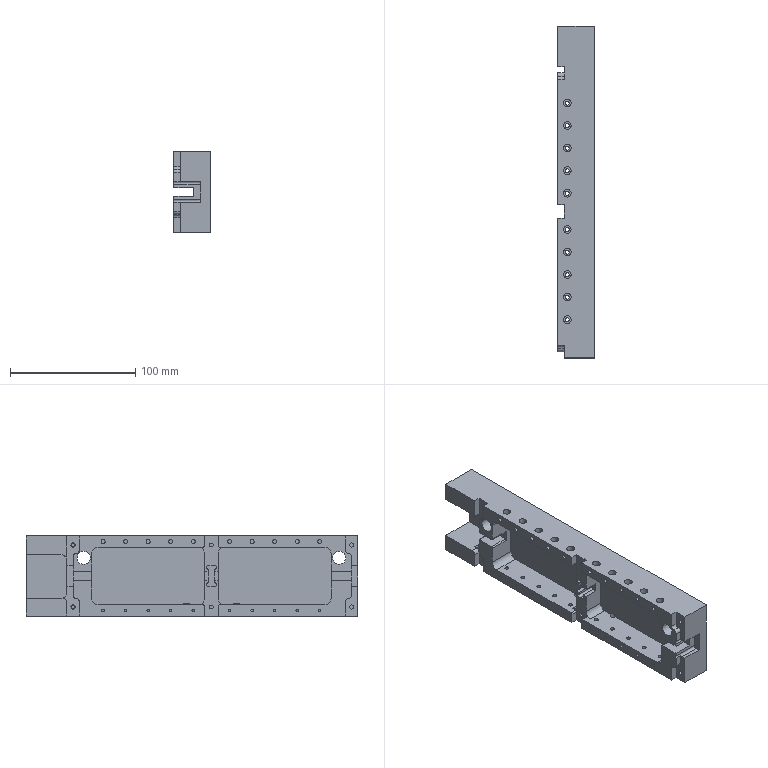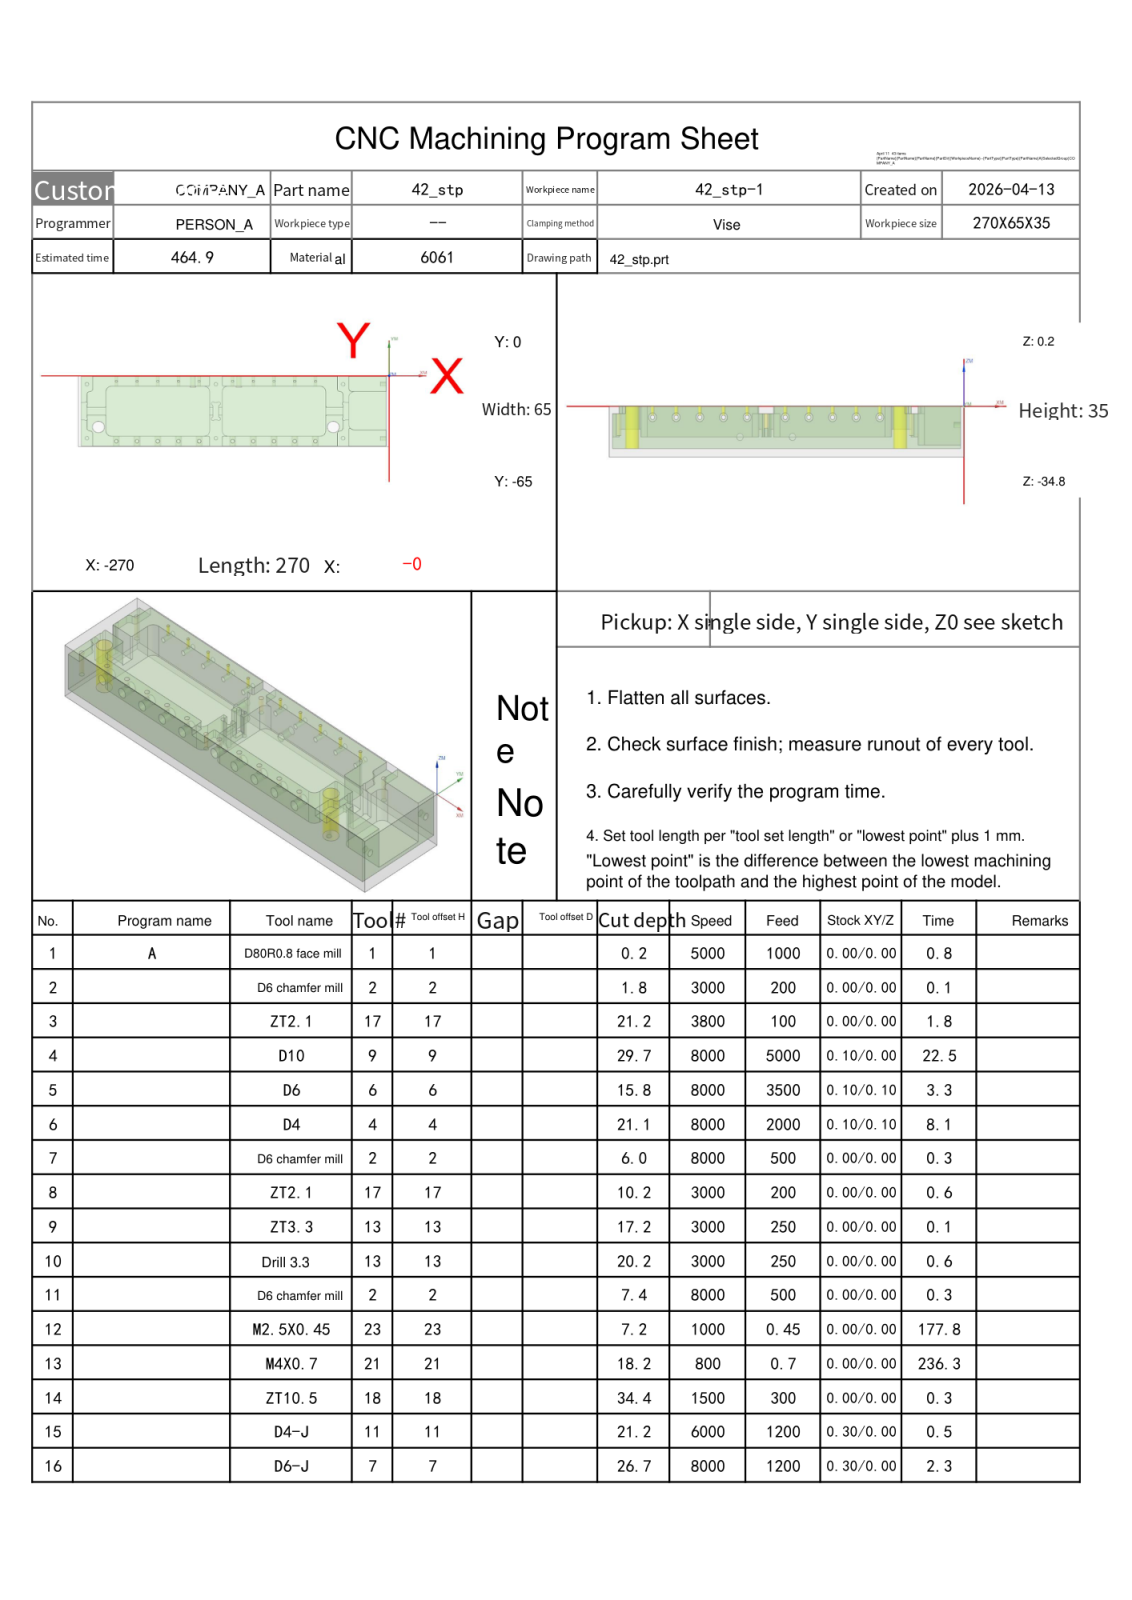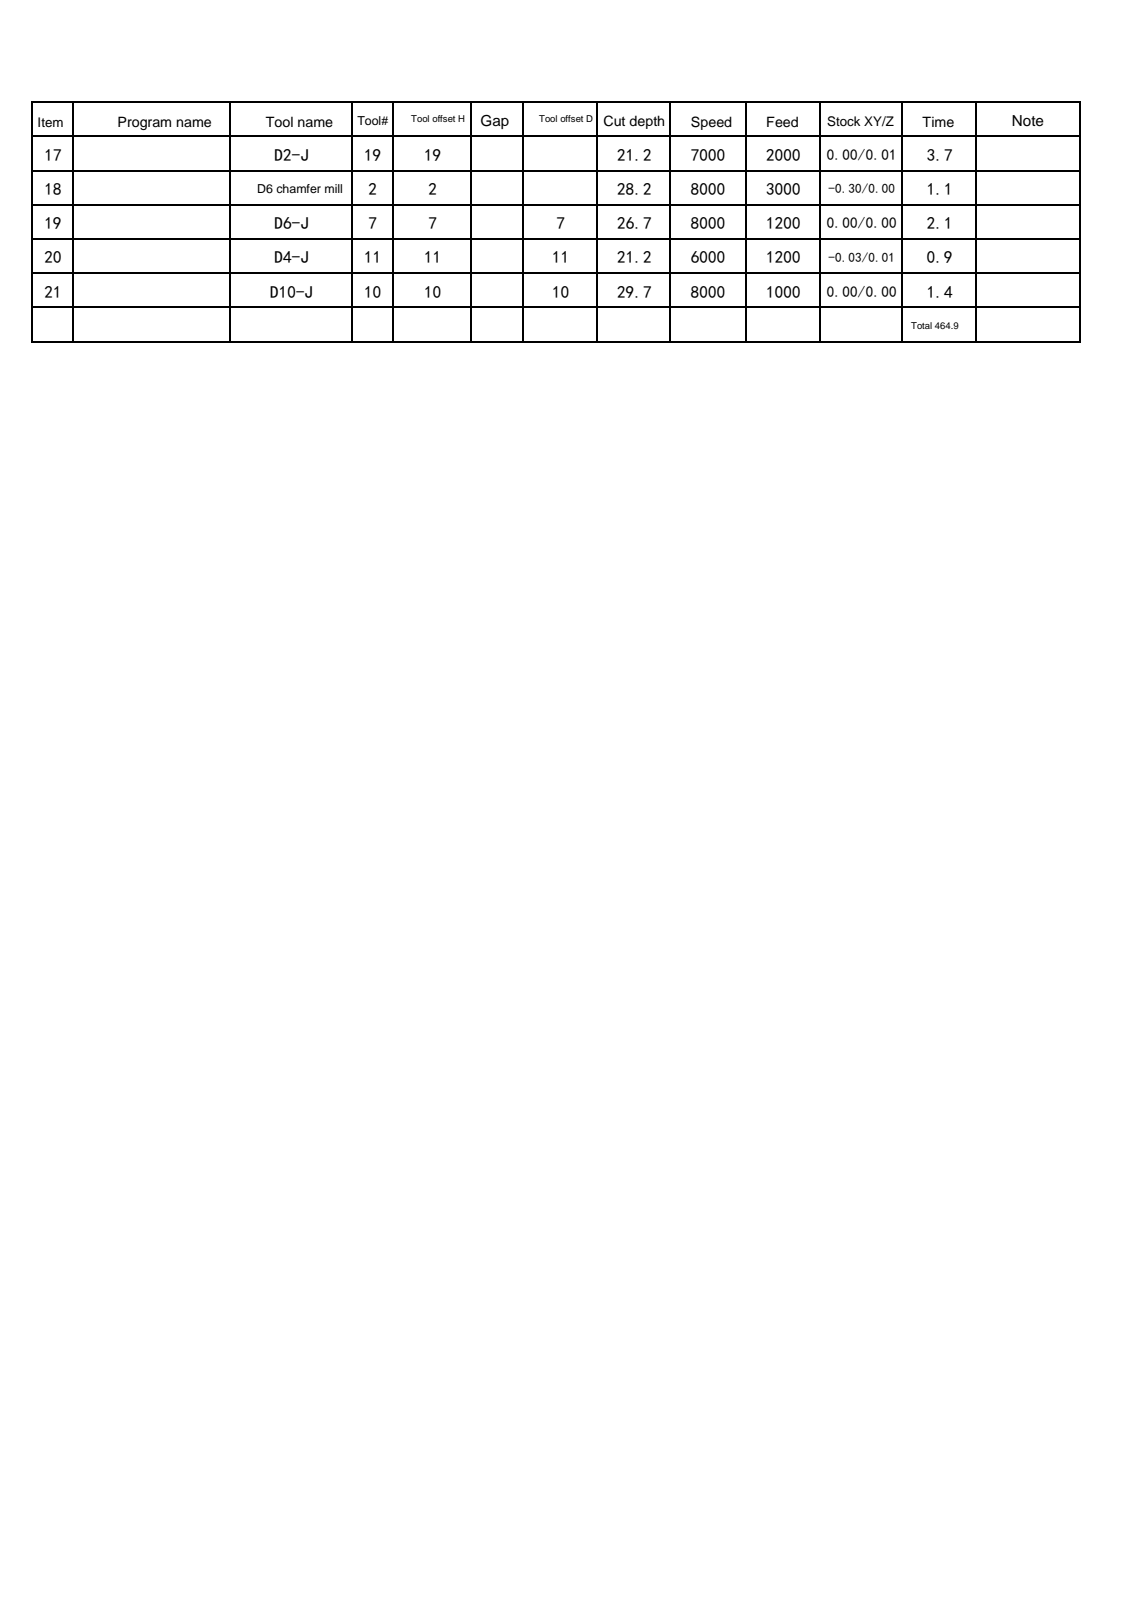NC program | NX | posted by the shop | part box 29 x 265 x 64 mm
Lines 6965 to 7681 of 41846:
N6 T04 M06
(D4  D=4. R=0. H=04 ce=0.10 di=0.10)
G00 G90 G54 X-150.05 Y-30.444 M03 S8000
G43 H04 Z20.
M08
Z-4.
G01 X-150.033 Y-26.941 Z-4.184 F2000.
X-149.901 Y-26.57 Z-4.204
X-151.099 Z-4.267
X-150.95 Y-27.178 Z-4.3
X-150.967 Y-38.059 Z-4.87
X-151.099 Y-38.43 Z-4.891
X-149.901 Z-4.954
X-150.033 Y-38.059 Z-4.974
X-150.05 Y-37.963 Z-4.979
Y-37.569 Z-5.
Y-27.431 Z-5.077
G02 X-149.901 Y-26.57 Z-5.084 I2.57 J0.0
G01 X-151.099 Z-5.093
G02 X-150.999 Y-26.93 Z-5.096 I-2.421 J-.861
X-150.95 Y-27.431 Z-5.099 I-2.521 J-.501
G01 Y-37.569 Z-5.176
G02 X-151.099 Y-38.43 Z-5.183 I-2.57 J0.0
G01 X-149.901 Z-5.192
G02 X-150.05 Y-37.569 Z-5.199 I2.421 J.861
G01 Y-27.431 Z-5.276
G02 X-149.901 Y-26.57 Z-5.282 I2.57 J0.0
G01 X-151.099 Z-5.291
G02 X-150.999 Y-26.93 Z-5.294 I-2.421 J-.861
X-150.95 Y-27.431 Z-5.298 I-2.521 J-.501
G01 Y-37.569 Z-5.375
G02 X-151.099 Y-38.43 Z-5.382 I-2.57 J0.0
G01 X-149.901 Z-5.391
G02 X-150.05 Y-37.569 Z-5.398 I2.421 J.861
G01 Y-27.431 Z-5.474
G02 X-149.901 Y-26.57 Z-5.481 I2.57 J0.0
G01 X-151.099 Z-5.49
G02 X-150.999 Y-26.93 Z-5.493 I-2.421 J-.861
X-150.95 Y-27.431 Z-5.497 I-2.521 J-.501
G01 Y-37.569 Z-5.574
G02 X-151.099 Y-38.43 Z-5.58 I-2.57 J0.0
G01 X-149.901 Z-5.59
G02 X-150.05 Y-37.569 Z-5.596 I2.421 J.861
G01 Y-27.431 Z-5.673
G02 X-149.901 Y-26.57 Z-5.68 I2.57 J0.0
G01 X-151.099 Z-5.689
G02 X-150.999 Y-26.93 Z-5.692 I-2.421 J-.861
X-150.95 Y-27.431 Z-5.696 I-2.521 J-.501
G01 Y-37.569 Z-5.773
G02 X-151.099 Y-38.43 Z-5.779 I-2.57 J0.0
G01 X-149.901 Z-5.788
G02 X-150.05 Y-37.569 Z-5.795 I2.421 J.861
G01 Y-27.431 Z-5.872
G02 X-149.901 Y-26.57 Z-5.879 I2.57 J0.0
G01 X-151.099 Z-5.888
G02 X-150.999 Y-26.93 Z-5.891 I-2.421 J-.861
X-150.95 Y-27.431 Z-5.894 I-2.521 J-.501
G01 Y-37.569 Z-5.971
G02 X-151.099 Y-38.43 Z-5.978 I-2.57 J0.0
G01 X-149.901 Z-5.987
G02 X-150.05 Y-37.569 Z-5.994 I2.421 J.861
G01 Y-27.431 Z-6.071
G02 X-149.901 Y-26.57 Z-6.077 I2.57 J0.0
G01 X-151.099 Z-6.086
G02 X-150.999 Y-26.93 Z-6.089 I-2.421 J-.861
X-150.95 Y-27.431 Z-6.093 I-2.521 J-.501
G01 Y-37.569 Z-6.17
G02 X-151.099 Y-38.43 Z-6.177 I-2.57 J0.0
G01 X-149.901 Z-6.186
G02 X-150.05 Y-37.569 Z-6.193 I2.421 J.861
G01 Y-27.431 Z-6.269
G02 X-149.901 Y-26.57 Z-6.276 I2.57 J0.0
G01 X-151.099 Z-6.285
G02 X-150.999 Y-26.93 Z-6.288 I-2.421 J-.861
X-150.95 Y-27.431 Z-6.292 I-2.521 J-.501
G01 Y-37.569 Z-6.369
G02 X-151.099 Y-38.43 Z-6.375 I-2.57 J0.0
G01 X-149.901 Z-6.385
G02 X-150.05 Y-37.569 Z-6.391 I2.421 J.861
G01 Y-27.431 Z-6.468
G02 X-149.901 Y-26.57 Z-6.475 I2.57 J0.0
G01 X-151.099 Z-6.484
G02 X-150.999 Y-26.93 Z-6.487 I-2.421 J-.861
X-150.95 Y-27.431 Z-6.491 I-2.521 J-.501
G01 Y-37.569 Z-6.568
G02 X-151.099 Y-38.43 Z-6.574 I-2.57 J0.0
G01 X-149.901 Z-6.583
G02 X-150.05 Y-37.569 Z-6.59 I2.421 J.861
G01 Y-27.431 Z-6.667
G02 X-149.901 Y-26.57 Z-6.674 I2.57 J0.0
G01 X-151.099 Z-6.683
G02 X-150.999 Y-26.93 Z-6.686 I-2.421 J-.861
X-150.95 Y-27.431 Z-6.689 I-2.521 J-.501
G01 Y-37.569 Z-6.766
G02 X-151.099 Y-38.43 Z-6.773 I-2.57 J0.0
G01 X-149.901 Z-6.782
G02 X-150.05 Y-37.569 Z-6.789 I2.421 J.861
G01 Y-27.431 Z-6.866
G02 X-149.901 Y-26.57 Z-6.872 I2.57 J0.0
G01 X-151.099 Z-6.881
G02 X-150.999 Y-26.93 Z-6.884 I-2.421 J-.861
X-150.95 Y-27.431 Z-6.888 I-2.521 J-.501
G01 Y-37.569 Z-6.965
G02 X-151.099 Y-38.43 Z-6.972 I-2.57 J0.0
G01 X-149.901 Z-6.981
G02 X-150.05 Y-37.569 Z-6.988 I2.421 J.861
G01 Y-27.431 Z-7.064
G02 X-149.901 Y-26.57 Z-7.071 I2.57 J0.0
G01 X-151.099 Z-7.08
G02 X-150.999 Y-26.93 Z-7.083 I-2.421 J-.861
X-150.95 Y-27.431 Z-7.087 I-2.521 J-.501
G01 Y-37.569 Z-7.164
G02 X-151.099 Y-38.43 Z-7.17 I-2.57 J0.0
G01 X-149.901 Z-7.18
G02 X-150.05 Y-37.569 Z-7.186 I2.421 J.861
G01 Y-27.431 Z-7.263
G02 X-149.901 Y-26.57 Z-7.27 I2.57 J0.0
G01 X-151.099 Z-7.279
G02 X-150.999 Y-26.93 Z-7.282 I-2.421 J-.861
X-150.95 Y-27.431 Z-7.286 I-2.521 J-.501
G01 Y-37.569 Z-7.363
G02 X-151.099 Y-38.43 Z-7.369 I-2.57 J0.0
G01 X-149.901 Z-7.378
G02 X-150.05 Y-37.569 Z-7.385 I2.421 J.861
G01 Y-27.431 Z-7.462
G02 X-149.901 Y-26.57 Z-7.469 I2.57 J0.0
G01 X-151.099 Z-7.478
G02 X-150.999 Y-26.93 Z-7.481 I-2.421 J-.861
X-150.95 Y-27.431 Z-7.484 I-2.521 J-.501
G01 Y-37.569 Z-7.561
G02 X-151.099 Y-38.43 Z-7.568 I-2.57 J0.0
G01 X-149.901 Z-7.577
G02 X-150.05 Y-37.569 Z-7.584 I2.421 J.861
G01 Y-27.431 Z-7.661
G02 X-149.901 Y-26.57 Z-7.667 I2.57 J0.0
G01 X-151.099 Z-7.676
G02 X-150.999 Y-26.93 Z-7.679 I-2.421 J-.861
X-150.95 Y-27.431 Z-7.683 I-2.521 J-.501
G01 Y-37.569 Z-7.76
G02 X-151.099 Y-38.43 Z-7.767 I-2.57 J0.0
G01 X-149.901 Z-7.776
G02 X-150.05 Y-37.569 Z-7.783 I2.421 J.861
G01 Y-27.431 Z-7.859
G02 X-149.901 Y-26.57 Z-7.866 I2.57 J0.0
G01 X-151.099 Z-7.875
G02 X-150.999 Y-26.93 Z-7.878 I-2.421 J-.861
X-150.95 Y-27.431 Z-7.882 I-2.521 J-.501
G01 Y-37.569 Z-7.959
G02 X-151.099 Y-38.43 Z-7.965 I-2.57 J0.0
G01 X-149.901 Z-7.975
G02 X-150.05 Y-37.569 Z-7.981 I2.421 J.861
G01 Y-27.431 Z-8.058
G02 X-149.901 Y-26.57 Z-8.065 I2.57 J0.0
G01 X-151.099 Z-8.074
G02 X-150.999 Y-26.93 Z-8.077 I-2.421 J-.861
X-150.95 Y-27.431 Z-8.081 I-2.521 J-.501
G01 Y-37.569 Z-8.158
G02 X-151.099 Y-38.43 Z-8.164 I-2.57 J0.0
G01 X-149.901 Z-8.173
G02 X-150.05 Y-37.569 Z-8.18 I2.421 J.861
G01 Y-27.431 Z-8.257
G02 X-149.901 Y-26.57 Z-8.264 I2.57 J0.0
G01 X-151.099 Z-8.273
G02 X-150.999 Y-26.93 Z-8.276 I-2.421 J-.861
X-150.95 Y-27.431 Z-8.279 I-2.521 J-.501
G01 Y-37.569 Z-8.356
G02 X-151.099 Y-38.43 Z-8.363 I-2.57 J0.0
G01 X-149.901 Z-8.372
G02 X-150.05 Y-37.569 Z-8.379 I2.421 J.861
G01 Y-27.431 Z-8.456
G02 X-149.901 Y-26.57 Z-8.462 I2.57 J0.0
G01 X-151.099 Z-8.471
G02 X-150.999 Y-26.93 Z-8.474 I-2.421 J-.861
X-150.95 Y-27.431 Z-8.478 I-2.521 J-.501
G01 Y-37.569 Z-8.555
G02 X-151.099 Y-38.43 Z-8.562 I-2.57 J0.0
G01 X-149.901 Z-8.571
G02 X-150.05 Y-37.569 Z-8.578 I2.421 J.861
G01 Y-27.431 Z-8.654
G02 X-149.901 Y-26.57 Z-8.661 I2.57 J0.0
G01 X-151.099 Z-8.67
G02 X-150.999 Y-26.93 Z-8.673 I-2.421 J-.861
X-150.95 Y-27.431 Z-8.677 I-2.521 J-.501
G01 Y-37.569 Z-8.754
G02 X-151.099 Y-38.43 Z-8.76 I-2.57 J0.0
G01 X-149.901 Z-8.77
G02 X-150.05 Y-37.569 Z-8.776 I2.421 J.861
G01 Y-27.431 Z-8.853
G02 X-149.901 Y-26.57 Z-8.86 I2.57 J0.0
G01 X-151.099 Z-8.869
G02 X-150.999 Y-26.93 Z-8.872 I-2.421 J-.861
X-150.95 Y-27.431 Z-8.876 I-2.521 J-.501
G01 Y-37.569 Z-8.953
G02 X-151.099 Y-38.43 Z-8.959 I-2.57 J0.0
G01 X-149.901 Z-8.968
G02 X-150.05 Y-37.569 Z-8.975 I2.421 J.861
G01 Y-27.431 Z-9.052
G02 X-149.901 Y-26.57 Z-9.059 I2.57 J0.0
G01 X-151.099 Z-9.068
G02 X-150.999 Y-26.93 Z-9.071 I-2.421 J-.861
X-150.95 Y-27.431 Z-9.074 I-2.521 J-.501
G01 Y-37.569 Z-9.151
G02 X-151.099 Y-38.43 Z-9.158 I-2.57 J0.0
G01 X-149.901 Z-9.167
G02 X-150.05 Y-37.569 Z-9.174 I2.421 J.861
G01 Y-27.431 Z-9.251
G02 X-149.901 Y-26.57 Z-9.257 I2.57 J0.0
G01 X-151.099 Z-9.266
G02 X-150.999 Y-26.93 Z-9.269 I-2.421 J-.861
X-150.95 Y-27.431 Z-9.273 I-2.521 J-.501
G01 Y-37.569 Z-9.35
G02 X-151.099 Y-38.43 Z-9.357 I-2.57 J0.0
G01 X-149.901 Z-9.366
G02 X-150.05 Y-37.569 Z-9.373 I2.421 J.861
G01 Y-27.431 Z-9.449
G02 X-149.901 Y-26.57 Z-9.456 I2.57 J0.0
G01 X-151.099 Z-9.465
G02 X-150.999 Y-26.93 Z-9.468 I-2.421 J-.861
X-150.95 Y-27.431 Z-9.472 I-2.521 J-.501
G01 Y-37.569 Z-9.549
G02 X-151.099 Y-38.43 Z-9.555 I-2.57 J0.0
G01 X-149.901 Z-9.565
G02 X-150.05 Y-37.569 Z-9.571 I2.421 J.861
G01 Y-27.431 Z-9.648
G02 X-149.901 Y-26.57 Z-9.655 I2.57 J0.0
G01 X-151.099 Z-9.664
G02 X-150.999 Y-26.93 Z-9.667 I-2.421 J-.861
X-150.95 Y-27.431 Z-9.671 I-2.521 J-.501
G01 Y-37.569 Z-9.748
G02 X-151.099 Y-38.43 Z-9.754 I-2.57 J0.0
G01 X-149.901 Z-9.763
G02 X-150.05 Y-37.569 Z-9.77 I2.421 J.861
G01 Y-27.431 Z-9.847
G02 X-149.901 Y-26.57 Z-9.854 I2.57 J0.0
G01 X-151.099 Z-9.863
G02 X-150.999 Y-26.93 Z-9.866 I-2.421 J-.861
X-150.95 Y-27.431 Z-9.869 I-2.521 J-.501
G01 Y-37.569 Z-9.946
G02 X-151.099 Y-38.43 Z-9.953 I-2.57 J0.0
G01 X-149.901 Z-9.962
G02 X-150.05 Y-37.569 Z-9.969 I2.421 J.861
G01 Y-27.431 Z-10.046
G02 X-149.901 Y-26.57 Z-10.052 I2.57 J0.0
G01 X-151.099 Z-10.061
G02 X-150.999 Y-26.93 Z-10.064 I-2.421 J-.861
X-150.95 Y-27.431 Z-10.068 I-2.521 J-.501
G01 Y-37.569 Z-10.145
G02 X-151.099 Y-38.43 Z-10.152 I-2.57 J0.0
G01 X-149.901 Z-10.161
G02 X-150.05 Y-37.569 Z-10.168 I2.421 J.861
G01 Y-27.431 Z-10.244
G02 X-149.901 Y-26.57 Z-10.251 I2.57 J0.0
G01 X-151.099 Z-10.26
G02 X-150.999 Y-26.93 Z-10.263 I-2.421 J-.861
X-150.95 Y-27.431 Z-10.267 I-2.521 J-.501
G01 Y-37.569 Z-10.344
G02 X-151.099 Y-38.43 Z-10.35 I-2.57 J0.0
G01 X-149.901 Z-10.36
G02 X-150.05 Y-37.569 Z-10.366 I2.421 J.861
G01 Y-27.431 Z-10.443
G02 X-149.901 Y-26.57 Z-10.45 I2.57 J0.0
G01 X-151.099 Z-10.459
G02 X-150.999 Y-26.93 Z-10.462 I-2.421 J-.861
X-150.95 Y-27.431 Z-10.466 I-2.521 J-.501
G01 Y-37.569 Z-10.543
G02 X-151.099 Y-38.43 Z-10.549 I-2.57 J0.0
G01 X-149.901 Z-10.558
G02 X-150.05 Y-37.569 Z-10.565 I2.421 J.861
G01 Y-27.431 Z-10.642
G02 X-149.901 Y-26.57 Z-10.649 I2.57 J0.0
G01 X-151.099 Z-10.658
G02 X-150.999 Y-26.93 Z-10.661 I-2.421 J-.861
X-150.95 Y-27.431 Z-10.664 I-2.521 J-.501
G01 Y-37.569 Z-10.741
G02 X-151.099 Y-38.43 Z-10.748 I-2.57 J0.0
G01 X-149.901 Z-10.757
G02 X-150.05 Y-37.569 Z-10.764 I2.421 J.861
G01 Y-27.431 Z-10.841
G02 X-149.901 Y-26.57 Z-10.847 I2.57 J0.0
G01 X-151.099 Z-10.856
G02 X-150.999 Y-26.93 Z-10.859 I-2.421 J-.861
X-150.95 Y-27.431 Z-10.863 I-2.521 J-.501
G01 Y-37.569 Z-10.94
G02 X-151.099 Y-38.43 Z-10.947 I-2.57 J0.0
G01 X-149.901 Z-10.956
G02 X-150.05 Y-37.569 Z-10.963 I2.421 J.861
G01 Y-27.431 Z-11.039
G02 X-149.901 Y-26.57 Z-11.046 I2.57 J0.0
G01 X-151.099 Z-11.055
G02 X-150.999 Y-26.93 Z-11.058 I-2.421 J-.861
X-150.95 Y-27.431 Z-11.062 I-2.521 J-.501
G01 Y-37.569 Z-11.139
G02 X-151.099 Y-38.43 Z-11.145 I-2.57 J0.0
G01 X-149.901 Z-11.155
G02 X-150.05 Y-37.569 Z-11.161 I2.421 J.861
G01 Y-27.431 Z-11.238
G02 X-149.901 Y-26.57 Z-11.245 I2.57 J0.0
G01 X-151.099 Z-11.254
G02 X-150.999 Y-26.93 Z-11.257 I-2.421 J-.861
X-150.95 Y-27.431 Z-11.261 I-2.521 J-.501
G01 Y-37.569 Z-11.338
G02 X-151.099 Y-38.43 Z-11.344 I-2.57 J0.0
G01 X-149.901 Z-11.353
G02 X-150.05 Y-37.569 Z-11.36 I2.421 J.861
G01 Y-27.431 Z-11.437
G02 X-149.901 Y-26.57 Z-11.444 I2.57 J0.0
G01 X-151.099 Z-11.453
G02 X-150.999 Y-26.93 Z-11.456 I-2.421 J-.861
X-150.95 Y-27.431 Z-11.459 I-2.521 J-.501
G01 Y-37.569 Z-11.536
G02 X-151.099 Y-38.43 Z-11.543 I-2.57 J0.0
G01 X-149.901 Z-11.552
G02 X-150.05 Y-37.569 Z-11.559 I2.421 J.861
G01 Y-27.431 Z-11.636
G02 X-149.901 Y-26.57 Z-11.642 I2.57 J0.0
G01 X-151.099 Z-11.651
G02 X-150.999 Y-26.93 Z-11.654 I-2.421 J-.861
X-150.95 Y-27.431 Z-11.658 I-2.521 J-.501
G01 Y-37.569 Z-11.735
G02 X-151.099 Y-38.43 Z-11.742 I-2.57 J0.0
G01 X-149.901 Z-11.751
G02 X-150.05 Y-37.569 Z-11.758 I2.421 J.861
G01 Y-27.431 Z-11.834
G02 X-149.901 Y-26.57 Z-11.841 I2.57 J0.0
G01 X-151.099 Z-11.85
G02 X-150.999 Y-26.93 Z-11.853 I-2.421 J-.861
X-150.95 Y-27.431 Z-11.857 I-2.521 J-.501
G01 Y-37.569 Z-11.934
G02 X-151.099 Y-38.43 Z-11.94 I-2.57 J0.0
G01 X-149.901 Z-11.95
G02 X-150.05 Y-37.569 Z-11.956 I2.421 J.861
G01 Y-27.431 Z-12.033
G02 X-149.901 Y-26.57 Z-12.04 I2.57 J0.0
G01 X-151.099 Z-12.049
G02 X-150.999 Y-26.93 Z-12.052 I-2.421 J-.861
X-150.95 Y-27.431 Z-12.056 I-2.521 J-.501
G01 Y-37.569 Z-12.133
G02 X-151.099 Y-38.43 Z-12.139 I-2.57 J0.0
G01 X-149.901 Z-12.148
G02 X-150.05 Y-37.569 Z-12.155 I2.421 J.861
G01 Y-27.431 Z-12.232
G02 X-149.901 Y-26.57 Z-12.239 I2.57 J0.0
G01 X-151.099 Z-12.248
G02 X-150.999 Y-26.93 Z-12.251 I-2.421 J-.861
X-150.95 Y-27.431 Z-12.254 I-2.521 J-.501
G01 Y-37.569 Z-12.331
G02 X-151.099 Y-38.43 Z-12.338 I-2.57 J0.0
G01 X-149.901 Z-12.347
G02 X-150.05 Y-37.569 Z-12.354 I2.421 J.861
G01 Y-27.431 Z-12.431
G02 X-149.901 Y-26.57 Z-12.437 I2.57 J0.0
G01 X-151.099 Z-12.446
G02 X-150.999 Y-26.93 Z-12.449 I-2.421 J-.861
X-150.95 Y-27.431 Z-12.453 I-2.521 J-.501
G01 Y-37.569 Z-12.53
G02 X-151.099 Y-38.43 Z-12.537 I-2.57 J0.0
G01 X-149.901 Z-12.546
G02 X-150.05 Y-37.569 Z-12.553 I2.421 J.861
G01 Y-27.431 Z-12.629
G02 X-149.901 Y-26.57 Z-12.636 I2.57 J0.0
G01 X-151.099 Z-12.645
G02 X-150.999 Y-26.93 Z-12.648 I-2.421 J-.861
X-150.95 Y-27.431 Z-12.652 I-2.521 J-.501
G01 Y-37.569 Z-12.729
G02 X-151.099 Y-38.43 Z-12.735 I-2.57 J0.0
G01 X-149.901 Z-12.745
G02 X-150.05 Y-37.569 Z-12.751 I2.421 J.861
G01 Y-27.431 Z-12.828
G02 X-149.901 Y-26.57 Z-12.835 I2.57 J0.0
G01 X-151.099 Z-12.844
G02 X-150.999 Y-26.93 Z-12.847 I-2.421 J-.861
X-150.95 Y-27.431 Z-12.851 I-2.521 J-.501
G01 Y-37.569 Z-12.928
G02 X-151.099 Y-38.43 Z-12.934 I-2.57 J0.0
G01 X-149.901 Z-12.943
G02 X-150.05 Y-37.569 Z-12.95 I2.421 J.861
G01 Y-27.431 Z-13.027
G02 X-149.901 Y-26.57 Z-13.034 I2.57 J0.0
G01 X-151.099 Z-13.043
G02 X-150.999 Y-26.93 Z-13.046 I-2.421 J-.861
X-150.95 Y-27.431 Z-13.049 I-2.521 J-.501
G01 Y-37.569 Z-13.126
G02 X-151.099 Y-38.43 Z-13.133 I-2.57 J0.0
G01 X-149.901 Z-13.142
G02 X-150.05 Y-37.569 Z-13.149 I2.421 J.861
G01 Y-27.431 Z-13.226
G02 X-149.901 Y-26.57 Z-13.232 I2.57 J0.0
G01 X-151.099 Z-13.241
G02 X-150.999 Y-26.93 Z-13.244 I-2.421 J-.861
X-150.95 Y-27.431 Z-13.248 I-2.521 J-.501
G01 Y-37.569 Z-13.325
G02 X-151.099 Y-38.43 Z-13.332 I-2.57 J0.0
G01 X-149.901 Z-13.341
G02 X-150.05 Y-37.569 Z-13.348 I2.421 J.861
G01 Y-27.431 Z-13.424
G02 X-149.901 Y-26.57 Z-13.431 I2.57 J0.0
G01 X-151.099 Z-13.44
G02 X-150.999 Y-26.93 Z-13.443 I-2.421 J-.861
X-150.95 Y-27.431 Z-13.447 I-2.521 J-.501
G01 Y-37.569 Z-13.524
G02 X-151.099 Y-38.43 Z-13.53 I-2.57 J0.0
G01 X-149.901 Z-13.54
G02 X-150.05 Y-37.569 Z-13.546 I2.421 J.861
G01 Y-27.431 Z-13.623
G02 X-149.901 Y-26.57 Z-13.63 I2.57 J0.0
G01 X-151.099 Z-13.639
G02 X-150.999 Y-26.93 Z-13.642 I-2.421 J-.861
X-150.95 Y-27.431 Z-13.646 I-2.521 J-.501
G01 Y-37.569 Z-13.723
G02 X-151.099 Y-38.43 Z-13.729 I-2.57 J0.0
G01 X-149.901 Z-13.738
G02 X-150.05 Y-37.569 Z-13.745 I2.421 J.861
G01 Y-27.431 Z-13.822
G02 X-149.901 Y-26.57 Z-13.829 I2.57 J0.0
G01 X-151.099 Z-13.838
G02 X-150.999 Y-26.93 Z-13.841 I-2.421 J-.861
X-150.95 Y-27.431 Z-13.844 I-2.521 J-.501
G01 Y-37.569 Z-13.921
G02 X-151.099 Y-38.43 Z-13.928 I-2.57 J0.0
G01 X-149.901 Z-13.937
G02 X-150.05 Y-37.569 Z-13.944 I2.421 J.861
G01 Y-27.431 Z-14.021
G02 X-149.901 Y-26.57 Z-14.027 I2.57 J0.0
G01 X-151.099 Z-14.036
G02 X-150.999 Y-26.93 Z-14.039 I-2.421 J-.861
X-150.95 Y-27.431 Z-14.043 I-2.521 J-.501
G01 Y-37.569 Z-14.12
G02 X-151.099 Y-38.43 Z-14.127 I-2.57 J0.0
G01 X-149.901 Z-14.136
G02 X-150.05 Y-37.569 Z-14.143 I2.421 J.861
G01 Y-27.431 Z-14.219
G02 X-149.901 Y-26.57 Z-14.226 I2.57 J0.0
G01 X-151.099 Z-14.235
G02 X-150.999 Y-26.93 Z-14.238 I-2.421 J-.861
X-150.95 Y-27.431 Z-14.242 I-2.521 J-.501
G01 Y-37.569 Z-14.319
G02 X-151.099 Y-38.43 Z-14.325 I-2.57 J0.0
G01 X-149.901 Z-14.335
G02 X-150.05 Y-37.569 Z-14.341 I2.421 J.861
G01 Y-27.431 Z-14.418
G02 X-149.901 Y-26.57 Z-14.425 I2.57 J0.0
G01 X-151.099 Z-14.434
G02 X-150.999 Y-26.93 Z-14.437 I-2.421 J-.861
X-150.95 Y-27.431 Z-14.441 I-2.521 J-.501
G01 Y-37.569 Z-14.518
G02 X-151.099 Y-38.43 Z-14.524 I-2.57 J0.0
G01 X-149.901 Z-14.533
G02 X-150.05 Y-37.569 Z-14.54 I2.421 J.861
G01 Y-27.431 Z-14.617
G02 X-149.901 Y-26.57 Z-14.624 I2.57 J0.0
G01 X-151.099 Z-14.633
G02 X-150.999 Y-26.93 Z-14.636 I-2.421 J-.861
X-150.95 Y-27.431 Z-14.639 I-2.521 J-.501
G01 Y-37.569 Z-14.716
G02 X-151.099 Y-38.43 Z-14.723 I-2.57 J0.0
G01 X-149.901 Z-14.732
G02 X-150.05 Y-37.569 Z-14.739 I2.421 J.861
G01 Y-27.431 Z-14.816
G02 X-149.901 Y-26.57 Z-14.822 I2.57 J0.0
G01 X-151.099 Z-14.831
G02 X-150.999 Y-26.93 Z-14.834 I-2.421 J-.861
X-150.95 Y-27.431 Z-14.838 I-2.521 J-.501
G01 Y-37.569 Z-14.915
G02 X-151.099 Y-38.43 Z-14.922 I-2.57 J0.0
G01 X-149.901 Z-14.931
G02 X-150.05 Y-37.569 Z-14.938 I2.421 J.861
G01 Y-27.431 Z-15.014
G02 X-149.901 Y-26.57 Z-15.021 I2.57 J0.0
G01 X-151.099 Z-15.03
G02 X-150.999 Y-26.93 Z-15.033 I-2.421 J-.861
X-150.95 Y-27.431 Z-15.037 I-2.521 J-.501
G01 Y-37.569 Z-15.114
G02 X-151.099 Y-38.43 Z-15.12 I-2.57 J0.0
G01 X-149.901 Z-15.13
G02 X-150.05 Y-37.569 Z-15.136 I2.421 J.861
G01 Y-27.431 Z-15.213
G02 X-149.901 Y-26.57 Z-15.22 I2.57 J0.0
G01 X-151.099 Z-15.229
G02 X-150.999 Y-26.93 Z-15.232 I-2.421 J-.861
X-150.95 Y-27.431 Z-15.236 I-2.521 J-.501
G01 Y-37.569 Z-15.313
G02 X-151.099 Y-38.43 Z-15.319 I-2.57 J0.0
G01 X-149.901 Z-15.328
G02 X-150.05 Y-37.569 Z-15.335 I2.421 J.861
G01 Y-27.431 Z-15.412
G02 X-149.901 Y-26.57 Z-15.419 I2.57 J0.0
G01 X-151.099 Z-15.428
G02 X-150.999 Y-26.93 Z-15.431 I-2.421 J-.861
X-150.95 Y-27.431 Z-15.434 I-2.521 J-.501
G01 Y-37.569 Z-15.511
G02 X-151.099 Y-38.43 Z-15.518 I-2.57 J0.0
G01 X-149.901 Z-15.527
G02 X-150.05 Y-37.569 Z-15.534 I2.421 J.861
G01 Y-27.431 Z-15.611
G02 X-149.901 Y-26.57 Z-15.617 I2.57 J0.0
G01 X-151.099 Z-15.626
G02 X-150.999 Y-26.93 Z-15.629 I-2.421 J-.861
X-150.95 Y-27.431 Z-15.633 I-2.521 J-.501
G01 Y-37.569 Z-15.71
G02 X-151.099 Y-38.43 Z-15.717 I-2.57 J0.0
G01 X-149.901 Z-15.726
G02 X-150.05 Y-37.569 Z-15.733 I2.421 J.861
G01 Y-27.431 Z-15.809
G02 X-149.901 Y-26.57 Z-15.816 I2.57 J0.0
G01 X-151.099 Z-15.825
G02 X-150.999 Y-26.93 Z-15.828 I-2.421 J-.861
X-150.95 Y-27.431 Z-15.832 I-2.521 J-.501
G01 Y-37.569 Z-15.909
G02 X-151.099 Y-38.43 Z-15.915 I-2.57 J0.0
G01 X-149.901 Z-15.925
G02 X-150.05 Y-37.569 Z-15.931 I2.421 J.861
G01 Y-27.431 Z-16.008
G02 X-149.901 Y-26.57 Z-16.015 I2.57 J0.0
G01 X-151.099 Z-16.024
G02 X-150.999 Y-26.93 Z-16.027 I-2.421 J-.861
X-150.95 Y-27.431 Z-16.031 I-2.521 J-.501
G01 Y-37.569 Z-16.108
G02 X-151.099 Y-38.43 Z-16.114 I-2.57 J0.0
G01 X-149.901 Z-16.123
G02 X-150.05 Y-37.569 Z-16.13 I2.421 J.861
G01 Y-27.431 Z-16.207
G02 X-149.901 Y-26.57 Z-16.214 I2.57 J0.0
G01 X-151.099 Z-16.223
G02 X-150.999 Y-26.93 Z-16.226 I-2.421 J-.861
X-150.95 Y-27.431 Z-16.229 I-2.521 J-.501
G01 Y-37.569 Z-16.306
G02 X-151.099 Y-38.43 Z-16.313 I-2.57 J0.0
G01 X-149.901 Z-16.322
G02 X-150.05 Y-37.569 Z-16.329 I2.421 J.861
G01 Y-27.431 Z-16.406
G02 X-149.901 Y-26.57 Z-16.412 I2.57 J0.0
G01 X-151.099 Z-16.421
G02 X-150.999 Y-26.93 Z-16.424 I-2.421 J-.861
X-150.95 Y-27.431 Z-16.428 I-2.521 J-.501
G01 Y-37.569 Z-16.505
G02 X-151.099 Y-38.43 Z-16.512 I-2.57 J0.0
G01 X-149.901 Z-16.521
G02 X-150.05 Y-37.569 Z-16.528 I2.421 J.861
G01 Y-27.431 Z-16.604
G02 X-149.901 Y-26.57 Z-16.611 I2.57 J0.0
G01 X-151.099 Z-16.62
G02 X-150.999 Y-26.93 Z-16.623 I-2.421 J-.861
X-150.95 Y-27.431 Z-16.627 I-2.521 J-.501
G01 Y-37.569 Z-16.704
G02 X-151.099 Y-38.43 Z-16.71 I-2.57 J0.0
G01 X-149.901 Z-16.72
G02 X-150.05 Y-37.569 Z-16.726 I2.421 J.861
G01 Y-27.431 Z-16.803
G02 X-149.901 Y-26.57 Z-16.81 I2.57 J0.0
G01 X-151.099 Z-16.819
G02 X-150.999 Y-26.93 Z-16.822 I-2.421 J-.861
X-150.95 Y-27.431 Z-16.826 I-2.521 J-.501
G01 Y-37.569 Z-16.903
G02 X-151.099 Y-38.43 Z-16.909 I-2.57 J0.0
G01 X-149.901 Z-16.918
G02 X-150.05 Y-37.569 Z-16.925 I2.421 J.861
G01 Y-27.431 Z-17.002
G02 X-149.901 Y-26.57 Z-17.009 I2.57 J0.0
G01 X-151.099 Z-17.018
G02 X-150.999 Y-26.93 Z-17.021 I-2.421 J-.861
X-150.95 Y-27.431 Z-17.024 I-2.521 J-.501
G01 Y-37.569 Z-17.101
G02 X-151.099 Y-38.43 Z-17.108 I-2.57 J0.0
G01 X-149.901 Z-17.117
G02 X-150.05 Y-37.569 Z-17.124 I2.421 J.861
G01 Y-27.431 Z-17.201
G02 X-149.901 Y-26.57 Z-17.207 I2.57 J0.0
G01 X-151.099 Z-17.216
G02 X-150.999 Y-26.93 Z-17.219 I-2.421 J-.861
X-150.95 Y-27.431 Z-17.223 I-2.521 J-.501
G01 Y-37.569 Z-17.3
G02 X-151.099 Y-38.43 Z-17.307 I-2.57 J0.0
G01 X-149.901 Z-17.316
G02 X-150.05 Y-37.569 Z-17.323 I2.421 J.861
G01 Y-27.431 Z-17.399
G02 X-149.901 Y-26.57 Z-17.406 I2.57 J0.0
G01 X-151.099 Z-17.415
G02 X-150.999 Y-26.93 Z-17.418 I-2.421 J-.861
X-150.95 Y-27.431 Z-17.422 I-2.521 J-.501
G01 Y-37.569 Z-17.499
G02 X-151.099 Y-38.43 Z-17.505 I-2.57 J0.0
G01 X-149.901 Z-17.515
G02 X-150.05 Y-37.569 Z-17.521 I2.421 J.861
G01 Y-27.431 Z-17.598
G02 X-149.901 Y-26.57 Z-17.605 I2.57 J0.0
G01 X-151.099 Z-17.614
G02 X-150.999 Y-26.93 Z-17.617 I-2.421 J-.861
X-150.95 Y-27.431 Z-17.621 I-2.521 J-.501
G01 Y-37.569 Z-17.698
G02 X-151.099 Y-38.43 Z-17.704 I-2.57 J0.0
G01 X-149.901 Z-17.713
G02 X-150.05 Y-37.569 Z-17.72 I2.421 J.861
G01 Y-27.431 Z-17.797
G02 X-149.901 Y-26.57 Z-17.804 I2.57 J0.0
G01 X-151.099 Z-17.813
G02 X-150.999 Y-26.93 Z-17.816 I-2.421 J-.861
X-150.95 Y-27.431 Z-17.819 I-2.521 J-.501
G01 Y-37.569 Z-17.896
G02 X-151.099 Y-38.43 Z-17.903 I-2.57 J0.0
G01 X-149.901 Z-17.912
G02 X-150.05 Y-37.569 Z-17.919 I2.421 J.861
G01 Y-27.431 Z-17.996
G02 X-149.901 Y-26.57 Z-18.002 I2.57 J0.0
G01 X-151.099 Z-18.011
G02 X-150.999 Y-26.93 Z-18.014 I-2.421 J-.861
X-150.95 Y-27.431 Z-18.018 I-2.521 J-.501
G01 Y-37.569 Z-18.095
G02 X-151.099 Y-38.43 Z-18.102 I-2.57 J0.0
G01 X-149.901 Z-18.111
G02 X-150.05 Y-37.569 Z-18.118 I2.421 J.861
G01 Y-27.431 Z-18.194
G02 X-149.901 Y-26.57 Z-18.201 I2.57 J0.0
G01 X-151.099 Z-18.21
G02 X-150.999 Y-26.93 Z-18.213 I-2.421 J-.861
X-150.95 Y-27.431 Z-18.217 I-2.521 J-.501
G01 Y-37.569 Z-18.294
G02 X-151.099 Y-38.43 Z-18.3 I-2.57 J0.0
G01 X-149.901 Z-18.31
G02 X-150.05 Y-37.569 Z-18.316 I2.421 J.861
G01 Y-27.431 Z-18.393
G02 X-149.901 Y-26.57 Z-18.4 I2.57 J0.0
G01 X-151.099 Z-18.409
G02 X-150.999 Y-26.93 Z-18.412 I-2.421 J-.861
X-150.95 Y-27.431 Z-18.416 I-2.521 J-.501
G01 Y-37.569 Z-18.493
G02 X-151.099 Y-38.43 Z-18.499 I-2.57 J0.0
G01 X-149.901 Z-18.508
G02 X-150.05 Y-37.569 Z-18.515 I2.421 J.861
G01 Y-27.431 Z-18.592
G02 X-149.901 Y-26.57 Z-18.599 I2.57 J0.0
G01 X-151.099 Z-18.608
G02 X-150.999 Y-26.93 Z-18.611 I-2.421 J-.861
X-150.95 Y-27.431 Z-18.614 I-2.521 J-.501
G01 Y-37.569 Z-18.691
G02 X-151.099 Y-38.43 Z-18.698 I-2.57 J0.0
G01 X-149.901 Z-18.707
G02 X-150.05 Y-37.569 Z-18.714 I2.421 J.861
G01 Y-27.431 Z-18.791
G02 X-149.901 Y-26.57 Z-18.797 I2.57 J0.0
G01 X-151.099 Z-18.806
G02 X-150.999 Y-26.93 Z-18.809 I-2.421 J-.861
X-150.95 Y-27.431 Z-18.813 I-2.521 J-.501
G01 Y-37.569 Z-18.89
G02 X-151.099 Y-38.43 Z-18.897 I-2.57 J0.0
G01 X-149.901 Z-18.906
G02 X-150.05 Y-37.569 Z-18.913 I2.421 J.861
G01 Y-27.431 Z-18.989
G02 X-149.901 Y-26.57 Z-18.996 I2.57 J0.0
G01 X-151.099 Z-19.005
G02 X-150.999 Y-26.93 Z-19.008 I-2.421 J-.861
X-150.95 Y-27.431 Z-19.012 I-2.521 J-.501
G01 Y-37.569 Z-19.089
G02 X-151.099 Y-38.43 Z-19.095 I-2.57 J0.0
G01 X-149.901 Z-19.105
G02 X-150.05 Y-37.569 Z-19.111 I2.421 J.861
G01 Y-27.431 Z-19.188
G02 X-149.901 Y-26.57 Z-19.195 I2.57 J0.0
G01 X-151.099 Z-19.204
G02 X-150.999 Y-26.93 Z-19.207 I-2.421 J-.861
X-150.95 Y-27.431 Z-19.211 I-2.521 J-.501
G01 Y-37.569 Z-19.288
G02 X-151.099 Y-38.43 Z-19.294 I-2.57 J0.0
G01 X-149.901 Z-19.303
G02 X-150.05 Y-37.569 Z-19.31 I2.421 J.861
G01 Y-27.431 Z-19.387
G02 X-149.901 Y-26.57 Z-19.394 I2.57 J0.0
G01 X-151.099 Z-19.403
G02 X-150.999 Y-26.93 Z-19.406 I-2.421 J-.861
X-150.95 Y-27.431 Z-19.409 I-2.521 J-.501
G01 Y-37.569 Z-19.486
G02 X-151.099 Y-38.43 Z-19.493 I-2.57 J0.0
G01 X-149.901 Z-19.502
G02 X-150.05 Y-37.569 Z-19.509 I2.421 J.861
G01 Y-27.431 Z-19.586
G02 X-149.901 Y-26.57 Z-19.592 I2.57 J0.0
G01 X-151.099 Z-19.601
G02 X-150.999 Y-26.93 Z-19.604 I-2.421 J-.861
X-150.95 Y-27.431 Z-19.608 I-2.521 J-.501
G01 Y-37.569 Z-19.685
G02 X-151.099 Y-38.43 Z-19.692 I-2.57 J0.0
G01 X-149.901 Z-19.701
G02 X-150.05 Y-37.569 Z-19.708 I2.421 J.861
G01 Y-27.431 Z-19.784
G02 X-149.901 Y-26.57 Z-19.791 I2.57 J0.0
G01 X-151.099 Z-19.8
G02 X-150.999 Y-26.93 Z-19.803 I-2.421 J-.861
X-150.95 Y-27.431 Z-19.807 I-2.521 J-.501
G01 Y-37.569 Z-19.884
G02 X-151.099 Y-38.43 Z-19.89 I-2.57 J0.0
G01 X-149.901 Z-19.9
G02 X-150.05 Y-37.569 Z-19.906 I2.421 J.861
G01 Y-27.431 Z-19.983
G02 X-149.901 Y-26.57 Z-19.99 I2.57 J0.0
G01 X-151.099 Z-19.999
G02 X-150.999 Y-26.93 Z-20.002 I-2.421 J-.861
X-150.95 Y-27.431 Z-20.006 I-2.521 J-.501
G01 Y-37.569 Z-20.083
G02 X-151.099 Y-38.43 Z-20.089 I-2.57 J0.0
G01 X-149.901 Z-20.098
G02 X-150.05 Y-37.569 Z-20.105 I2.421 J.861
G01 Y-27.431 Z-20.182
G02 X-149.901 Y-26.57 Z-20.189 I2.57 J0.0
G01 X-151.099 Z-20.198
G02 X-150.999 Y-26.93 Z-20.201 I-2.421 J-.861
X-150.95 Y-27.431 Z-20.204 I-2.521 J-.501
G01 Y-37.569 Z-20.281
G02 X-151.099 Y-38.43 Z-20.288 I-2.57 J0.0
G01 X-149.901 Z-20.297
G02 X-150.05 Y-37.569 Z-20.304 I2.421 J.861
G01 Y-27.431 Z-20.381
G02 X-149.901 Y-26.57 Z-20.387 I2.57 J0.0
G01 X-151.099 Z-20.396
G02 X-150.999 Y-26.93 Z-20.399 I-2.421 J-.861
X-150.95 Y-27.431 Z-20.403 I-2.521 J-.501
G01 Y-37.569 Z-20.48
G02 X-151.099 Y-38.43 Z-20.487 I-2.57 J0.0
G01 X-149.901 Z-20.496